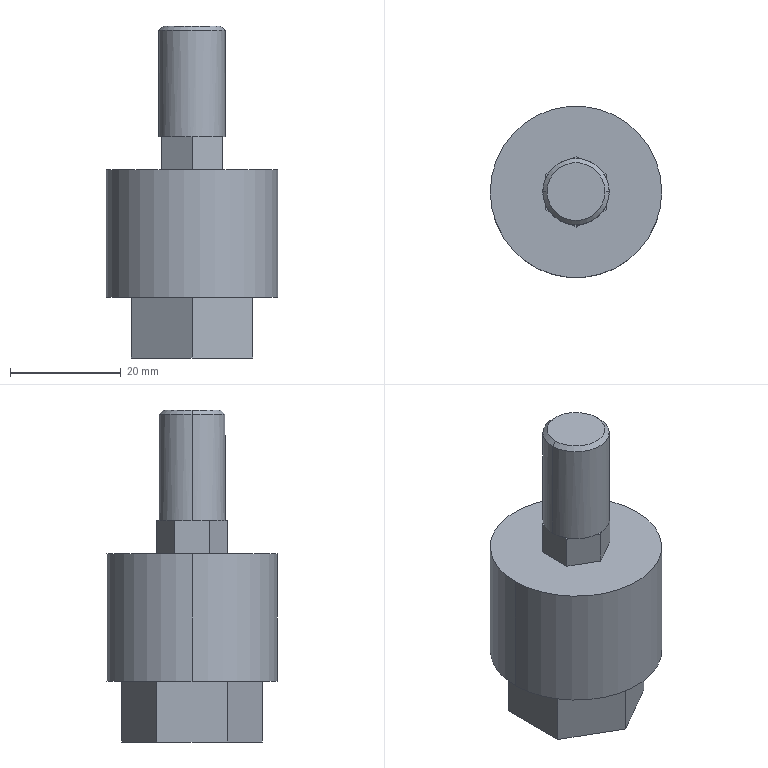Part | STEP file | JA40_12_125_JA40-12-125 | 1 solid | 39 faces | box 31 x 31 x 60 mm | volume 23685 mm3 | plane 29 | cylinder 6 | cone 4 | commonest cylinder face diameters 10.647 x2 12 x2 31 x2
STEP:
#1=CARTESIAN_POINT('',(-6.,0.,59.233));
#2=VERTEX_POINT('',#1);
#3=CARTESIAN_POINT('',(6.,0.,59.233));
#4=VERTEX_POINT('',#3);
#5=CARTESIAN_POINT('',(0.,0.,59.233));
#6=DIRECTION('',(0.,0.,-1.));
#7=DIRECTION('',(-1.,0.,0.));
#8=AXIS2_PLACEMENT_3D('',#5,#6,#7);
#9=CIRCLE('',#8,6.);
#10=EDGE_CURVE('',#2,#4,#9,.T.);
#11=ORIENTED_EDGE('',*,*,#10,.T.);
#12=CARTESIAN_POINT('',(6.,0.,40.));
#13=VERTEX_POINT('',#12);
#14=CARTESIAN_POINT('',(6.,0.,40.));
#15=DIRECTION('',(0.,0.,-1.));
#16=VECTOR('',#15,1000.);
#17=LINE('',#14,#16);
#18=EDGE_CURVE('',#4,#13,#17,.T.);
#19=ORIENTED_EDGE('',*,*,#18,.T.);
#20=CARTESIAN_POINT('',(5.5,2.398,40.));
#21=VERTEX_POINT('',#20);
#22=CARTESIAN_POINT('',(0.,0.,40.));
#23=DIRECTION('',(0.,0.,-1.));
#24=DIRECTION('',(-1.,0.,0.));
#25=AXIS2_PLACEMENT_3D('',#22,#23,#24);
#26=CIRCLE('',#25,6.);
#27=EDGE_CURVE('',#21,#13,#26,.T.);
#28=ORIENTED_EDGE('',*,*,#27,.F.);
#29=CARTESIAN_POINT('',(4.827,3.564,40.));
#30=VERTEX_POINT('',#29);
#31=CARTESIAN_POINT('',(0.,0.,40.));
#32=DIRECTION('',(0.,0.,-1.));
#33=DIRECTION('',(-1.,0.,0.));
#34=AXIS2_PLACEMENT_3D('',#31,#32,#33);
#35=CIRCLE('',#34,6.);
#36=EDGE_CURVE('',#30,#21,#35,.T.);
#37=ORIENTED_EDGE('',*,*,#36,.F.);
#38=CARTESIAN_POINT('',(0.6733,5.962,40.));
#39=VERTEX_POINT('',#38);
#40=CARTESIAN_POINT('',(0.,0.,40.));
#41=DIRECTION('',(0.,0.,-1.));
#42=DIRECTION('',(-1.,0.,0.));
#43=AXIS2_PLACEMENT_3D('',#40,#41,#42);
#44=CIRCLE('',#43,6.);
#45=EDGE_CURVE('',#39,#30,#44,.T.);
#46=ORIENTED_EDGE('',*,*,#45,.F.);
#47=CARTESIAN_POINT('',(-0.6733,5.962,40.));
#48=VERTEX_POINT('',#47);
#49=CARTESIAN_POINT('',(0.,0.,40.));
#50=DIRECTION('',(0.,0.,-1.));
#51=DIRECTION('',(-1.,0.,0.));
#52=AXIS2_PLACEMENT_3D('',#49,#50,#51);
#53=CIRCLE('',#52,6.);
#54=EDGE_CURVE('',#48,#39,#53,.T.);
#55=ORIENTED_EDGE('',*,*,#54,.F.);
#56=CARTESIAN_POINT('',(-4.827,3.564,40.));
#57=VERTEX_POINT('',#56);
#58=CARTESIAN_POINT('',(0.,0.,40.));
#59=DIRECTION('',(0.,0.,-1.));
#60=DIRECTION('',(-1.,0.,0.));
#61=AXIS2_PLACEMENT_3D('',#58,#59,#60);
#62=CIRCLE('',#61,6.);
#63=EDGE_CURVE('',#57,#48,#62,.T.);
#64=ORIENTED_EDGE('',*,*,#63,.F.);
#65=CARTESIAN_POINT('',(-5.5,2.398,40.));
#66=VERTEX_POINT('',#65);
#67=CARTESIAN_POINT('',(0.,0.,40.));
#68=DIRECTION('',(0.,0.,-1.));
#69=DIRECTION('',(-1.,0.,0.));
#70=AXIS2_PLACEMENT_3D('',#67,#68,#69);
#71=CIRCLE('',#70,6.);
#72=EDGE_CURVE('',#66,#57,#71,.T.);
#73=ORIENTED_EDGE('',*,*,#72,.F.);
#74=CARTESIAN_POINT('',(-6.,0.,40.));
#75=VERTEX_POINT('',#74);
#76=CARTESIAN_POINT('',(0.,0.,40.));
#77=DIRECTION('',(0.,0.,-1.));
#78=DIRECTION('',(-1.,0.,0.));
#79=AXIS2_PLACEMENT_3D('',#76,#77,#78);
#80=CIRCLE('',#79,6.);
#81=EDGE_CURVE('',#75,#66,#80,.T.);
#82=ORIENTED_EDGE('',*,*,#81,.F.);
#83=CARTESIAN_POINT('',(-6.,0.,40.));
#84=DIRECTION('',(0.,0.,-1.));
#85=VECTOR('',#84,1000.);
#86=LINE('',#83,#85);
#87=EDGE_CURVE('',#2,#75,#86,.T.);
#88=ORIENTED_EDGE('',*,*,#87,.F.);
#89=EDGE_LOOP('',(#11,#19,#28,#37,#46,#55,#64,#73,#82,#88));
#90=FACE_OUTER_BOUND('',#89,.T.);
#91=CARTESIAN_POINT('',(0.,0.,40.));
#92=DIRECTION('',(0.,0.,-1.));
#93=DIRECTION('',(-1.,0.,0.));
#94=AXIS2_PLACEMENT_3D('',#91,#92,#93);
#95=CYLINDRICAL_SURFACE('',#94,6.);
#96=ADVANCED_FACE('',(#90),#95,.T.);
#97=CARTESIAN_POINT('',(-5.233,0.,60.));
#98=VERTEX_POINT('',#97);
#99=CARTESIAN_POINT('',(5.233,0.,60.));
#100=VERTEX_POINT('',#99);
#101=CARTESIAN_POINT('',(0.,0.,60.));
#102=DIRECTION('',(0.,0.,-1.));
#103=DIRECTION('',(-1.,0.,0.));
#104=AXIS2_PLACEMENT_3D('',#101,#102,#103);
#105=CIRCLE('',#104,5.233);
#106=EDGE_CURVE('',#98,#100,#105,.T.);
#107=ORIENTED_EDGE('',*,*,#106,.T.);
#108=CARTESIAN_POINT('',(6.,0.,59.233));
#109=DIRECTION('',(0.7071,0.,-0.7071));
#110=VECTOR('',#109,1000.);
#111=LINE('',#108,#110);
#112=EDGE_CURVE('',#100,#4,#111,.T.);
#113=ORIENTED_EDGE('',*,*,#112,.T.);
#114=ORIENTED_EDGE('',*,*,#10,.F.);
#115=CARTESIAN_POINT('',(-6.,0.,59.233));
#116=DIRECTION('',(-0.7071,0.,-0.7071));
#117=VECTOR('',#116,1000.);
#118=LINE('',#115,#117);
#119=EDGE_CURVE('',#98,#2,#118,.T.);
#120=ORIENTED_EDGE('',*,*,#119,.F.);
#121=EDGE_LOOP('',(#107,#113,#114,#120));
#122=FACE_OUTER_BOUND('',#121,.T.);
#123=CARTESIAN_POINT('',(0.,0.,59.233));
#124=DIRECTION('',(0.,0.,-1.));
#125=DIRECTION('',(-1.,0.,0.));
#126=AXIS2_PLACEMENT_3D('',#123,#124,#125);
#127=CONICAL_SURFACE('',#126,6.,0.7854);
#128=ADVANCED_FACE('',(#122),#127,.T.);
#129=CARTESIAN_POINT('',(5.324,0.,0.6765));
#130=VERTEX_POINT('',#129);
#131=CARTESIAN_POINT('',(-5.324,0.,0.6765));
#132=VERTEX_POINT('',#131);
#133=CARTESIAN_POINT('',(0.,0.,0.6765));
#134=DIRECTION('',(0.,0.,-1.));
#135=DIRECTION('',(-1.,0.,0.));
#136=AXIS2_PLACEMENT_3D('',#133,#134,#135);
#137=CIRCLE('',#136,5.324);
#138=EDGE_CURVE('',#130,#132,#137,.T.);
#139=ORIENTED_EDGE('',*,*,#138,.F.);
#140=CARTESIAN_POINT('',(6.,0.,0.));
#141=VERTEX_POINT('',#140);
#142=CARTESIAN_POINT('',(5.324,0.,0.6765));
#143=DIRECTION('',(0.7071,0.,-0.7071));
#144=VECTOR('',#143,1000.);
#145=LINE('',#142,#144);
#146=EDGE_CURVE('',#130,#141,#145,.T.);
#147=ORIENTED_EDGE('',*,*,#146,.T.);
#148=CARTESIAN_POINT('',(-6.,0.,0.));
#149=VERTEX_POINT('',#148);
#150=CARTESIAN_POINT('',(0.,0.,0.));
#151=DIRECTION('',(0.,0.,-1.));
#152=DIRECTION('',(-1.,0.,0.));
#153=AXIS2_PLACEMENT_3D('',#150,#151,#152);
#154=CIRCLE('',#153,6.);
#155=EDGE_CURVE('',#141,#149,#154,.T.);
#156=ORIENTED_EDGE('',*,*,#155,.T.);
#157=CARTESIAN_POINT('',(-5.324,0.,0.6765));
#158=DIRECTION('',(-0.7071,0.,-0.7071));
#159=VECTOR('',#158,1000.);
#160=LINE('',#157,#159);
#161=EDGE_CURVE('',#132,#149,#160,.T.);
#162=ORIENTED_EDGE('',*,*,#161,.F.);
#163=EDGE_LOOP('',(#139,#147,#156,#162));
#164=FACE_OUTER_BOUND('',#163,.T.);
#165=CARTESIAN_POINT('',(0.,0.,0.6765));
#166=DIRECTION('',(0.,0.,-1.));
#167=DIRECTION('',(-1.,0.,0.));
#168=AXIS2_PLACEMENT_3D('',#165,#166,#167);
#169=CONICAL_SURFACE('',#168,5.324,0.7854);
#170=ADVANCED_FACE('',(#164),#169,.F.);
#171=CARTESIAN_POINT('',(5.324,0.,13.));
#172=VERTEX_POINT('',#171);
#173=CARTESIAN_POINT('',(-5.324,0.,13.));
#174=VERTEX_POINT('',#173);
#175=CARTESIAN_POINT('',(0.,0.,13.));
#176=DIRECTION('',(0.,0.,-1.));
#177=DIRECTION('',(-1.,0.,0.));
#178=AXIS2_PLACEMENT_3D('',#175,#176,#177);
#179=CIRCLE('',#178,5.324);
#180=EDGE_CURVE('',#172,#174,#179,.T.);
#181=ORIENTED_EDGE('',*,*,#180,.F.);
#182=CARTESIAN_POINT('',(5.324,0.,0.));
#183=DIRECTION('',(0.,0.,-1.));
#184=VECTOR('',#183,1000.);
#185=LINE('',#182,#184);
#186=EDGE_CURVE('',#172,#130,#185,.T.);
#187=ORIENTED_EDGE('',*,*,#186,.T.);
#188=ORIENTED_EDGE('',*,*,#138,.T.);
#189=CARTESIAN_POINT('',(-5.324,0.,0.));
#190=DIRECTION('',(0.,0.,-1.));
#191=VECTOR('',#190,1000.);
#192=LINE('',#189,#191);
#193=EDGE_CURVE('',#174,#132,#192,.T.);
#194=ORIENTED_EDGE('',*,*,#193,.F.);
#195=EDGE_LOOP('',(#181,#187,#188,#194));
#196=FACE_OUTER_BOUND('',#195,.T.);
#197=CARTESIAN_POINT('',(0.,0.,0.));
#198=DIRECTION('',(0.,0.,-1.));
#199=DIRECTION('',(-1.,0.,0.));
#200=AXIS2_PLACEMENT_3D('',#197,#198,#199);
#201=CYLINDRICAL_SURFACE('',#200,5.324);
#202=ADVANCED_FACE('',(#196),#201,.F.);
#203=CARTESIAN_POINT('',(-15.5,0.,34.));
#204=VERTEX_POINT('',#203);
#205=CARTESIAN_POINT('',(15.5,0.,34.));
#206=VERTEX_POINT('',#205);
#207=CARTESIAN_POINT('',(0.,0.,34.));
#208=DIRECTION('',(0.,0.,-1.));
#209=DIRECTION('',(-1.,0.,0.));
#210=AXIS2_PLACEMENT_3D('',#207,#208,#209);
#211=CIRCLE('',#210,15.5);
#212=EDGE_CURVE('',#204,#206,#211,.T.);
#213=ORIENTED_EDGE('',*,*,#212,.T.);
#214=CARTESIAN_POINT('',(15.5,0.,11.));
#215=VERTEX_POINT('',#214);
#216=CARTESIAN_POINT('',(15.5,0.,0.));
#217=DIRECTION('',(0.,0.,-1.));
#218=VECTOR('',#217,1000.);
#219=LINE('',#216,#218);
#220=EDGE_CURVE('',#206,#215,#219,.T.);
#221=ORIENTED_EDGE('',*,*,#220,.T.);
#222=CARTESIAN_POINT('',(-15.5,0.,11.));
#223=VERTEX_POINT('',#222);
#224=CARTESIAN_POINT('',(0.,0.,11.));
#225=DIRECTION('',(0.,0.,-1.));
#226=DIRECTION('',(-1.,0.,0.));
#227=AXIS2_PLACEMENT_3D('',#224,#225,#226);
#228=CIRCLE('',#227,15.5);
#229=EDGE_CURVE('',#223,#215,#228,.T.);
#230=ORIENTED_EDGE('',*,*,#229,.F.);
#231=CARTESIAN_POINT('',(-15.5,0.,0.));
#232=DIRECTION('',(0.,0.,-1.));
#233=VECTOR('',#232,1000.);
#234=LINE('',#231,#233);
#235=EDGE_CURVE('',#204,#223,#234,.T.);
#236=ORIENTED_EDGE('',*,*,#235,.F.);
#237=EDGE_LOOP('',(#213,#221,#230,#236));
#238=FACE_OUTER_BOUND('',#237,.T.);
#239=CARTESIAN_POINT('',(0.,0.,0.));
#240=DIRECTION('',(0.,0.,-1.));
#241=DIRECTION('',(-1.,0.,0.));
#242=AXIS2_PLACEMENT_3D('',#239,#240,#241);
#243=CYLINDRICAL_SURFACE('',#242,15.5);
#244=ADVANCED_FACE('',(#238),#243,.T.);
#245=CARTESIAN_POINT('',(-5.5,3.175,40.));
#246=VERTEX_POINT('',#245);
#247=CARTESIAN_POINT('',(-5.5,3.175,40.));
#248=DIRECTION('',(0.,-1.,0.));
#249=VECTOR('',#248,1000.);
#250=LINE('',#247,#249);
#251=EDGE_CURVE('',#246,#66,#250,.T.);
#252=ORIENTED_EDGE('',*,*,#251,.T.);
#253=ORIENTED_EDGE('',*,*,#72,.T.);
#254=CARTESIAN_POINT('',(0.,6.351,40.));
#255=DIRECTION('',(-0.866,-0.5,0.));
#256=VECTOR('',#255,1000.);
#257=LINE('',#254,#256);
#258=EDGE_CURVE('',#57,#246,#257,.T.);
#259=ORIENTED_EDGE('',*,*,#258,.T.);
#260=EDGE_LOOP('',(#252,#253,#259));
#261=FACE_OUTER_BOUND('',#260,.T.);
#262=CARTESIAN_POINT('',(-5.5,3.175,40.));
#263=DIRECTION('',(0.,0.,1.));
#264=DIRECTION('',(1.,0.,0.));
#265=AXIS2_PLACEMENT_3D('',#262,#263,#264);
#266=PLANE('',#265);
#267=ADVANCED_FACE('',(#261),#266,.T.);
#268=CARTESIAN_POINT('',(0.,6.351,40.));
#269=VERTEX_POINT('',#268);
#270=CARTESIAN_POINT('',(0.,6.351,40.));
#271=DIRECTION('',(-0.866,-0.5,0.));
#272=VECTOR('',#271,1000.);
#273=LINE('',#270,#272);
#274=EDGE_CURVE('',#269,#48,#273,.T.);
#275=ORIENTED_EDGE('',*,*,#274,.T.);
#276=ORIENTED_EDGE('',*,*,#54,.T.);
#277=CARTESIAN_POINT('',(5.5,3.175,40.));
#278=DIRECTION('',(-0.866,0.5,0.));
#279=VECTOR('',#278,1000.);
#280=LINE('',#277,#279);
#281=EDGE_CURVE('',#39,#269,#280,.T.);
#282=ORIENTED_EDGE('',*,*,#281,.T.);
#283=EDGE_LOOP('',(#275,#276,#282));
#284=FACE_OUTER_BOUND('',#283,.T.);
#285=CARTESIAN_POINT('',(-5.5,3.175,40.));
#286=DIRECTION('',(0.,0.,1.));
#287=DIRECTION('',(1.,0.,0.));
#288=AXIS2_PLACEMENT_3D('',#285,#286,#287);
#289=PLANE('',#288);
#290=ADVANCED_FACE('',(#284),#289,.T.);
#291=CARTESIAN_POINT('',(5.5,3.175,40.));
#292=VERTEX_POINT('',#291);
#293=CARTESIAN_POINT('',(5.5,3.175,40.));
#294=DIRECTION('',(-0.866,0.5,0.));
#295=VECTOR('',#294,1000.);
#296=LINE('',#293,#295);
#297=EDGE_CURVE('',#292,#30,#296,.T.);
#298=ORIENTED_EDGE('',*,*,#297,.T.);
#299=ORIENTED_EDGE('',*,*,#36,.T.);
#300=CARTESIAN_POINT('',(5.5,-3.175,40.));
#301=DIRECTION('',(0.,1.,0.));
#302=VECTOR('',#301,1000.);
#303=LINE('',#300,#302);
#304=EDGE_CURVE('',#21,#292,#303,.T.);
#305=ORIENTED_EDGE('',*,*,#304,.T.);
#306=EDGE_LOOP('',(#298,#299,#305));
#307=FACE_OUTER_BOUND('',#306,.T.);
#308=CARTESIAN_POINT('',(-5.5,3.175,40.));
#309=DIRECTION('',(0.,0.,1.));
#310=DIRECTION('',(1.,0.,0.));
#311=AXIS2_PLACEMENT_3D('',#308,#309,#310);
#312=PLANE('',#311);
#313=ADVANCED_FACE('',(#307),#312,.T.);
#314=CARTESIAN_POINT('',(5.5,-3.175,40.));
#315=VERTEX_POINT('',#314);
#316=CARTESIAN_POINT('',(5.5,-2.398,40.));
#317=VERTEX_POINT('',#316);
#318=CARTESIAN_POINT('',(5.5,-3.175,40.));
#319=DIRECTION('',(0.,1.,0.));
#320=VECTOR('',#319,1000.);
#321=LINE('',#318,#320);
#322=EDGE_CURVE('',#315,#317,#321,.T.);
#323=ORIENTED_EDGE('',*,*,#322,.T.);
#324=CARTESIAN_POINT('',(4.827,-3.564,40.));
#325=VERTEX_POINT('',#324);
#326=CARTESIAN_POINT('',(0.,0.,40.));
#327=DIRECTION('',(0.,0.,-1.));
#328=DIRECTION('',(-1.,0.,0.));
#329=AXIS2_PLACEMENT_3D('',#326,#327,#328);
#330=CIRCLE('',#329,6.);
#331=EDGE_CURVE('',#317,#325,#330,.T.);
#332=ORIENTED_EDGE('',*,*,#331,.T.);
#333=CARTESIAN_POINT('',(0.,-6.351,40.));
#334=DIRECTION('',(0.866,0.5,0.));
#335=VECTOR('',#334,1000.);
#336=LINE('',#333,#335);
#337=EDGE_CURVE('',#325,#315,#336,.T.);
#338=ORIENTED_EDGE('',*,*,#337,.T.);
#339=EDGE_LOOP('',(#323,#332,#338));
#340=FACE_OUTER_BOUND('',#339,.T.);
#341=CARTESIAN_POINT('',(-5.5,3.175,40.));
#342=DIRECTION('',(0.,0.,1.));
#343=DIRECTION('',(1.,0.,0.));
#344=AXIS2_PLACEMENT_3D('',#341,#342,#343);
#345=PLANE('',#344);
#346=ADVANCED_FACE('',(#340),#345,.T.);
#347=CARTESIAN_POINT('',(0.,-6.351,40.));
#348=VERTEX_POINT('',#347);
#349=CARTESIAN_POINT('',(0.6733,-5.962,40.));
#350=VERTEX_POINT('',#349);
#351=CARTESIAN_POINT('',(0.,-6.351,40.));
#352=DIRECTION('',(0.866,0.5,0.));
#353=VECTOR('',#352,1000.);
#354=LINE('',#351,#353);
#355=EDGE_CURVE('',#348,#350,#354,.T.);
#356=ORIENTED_EDGE('',*,*,#355,.T.);
#357=CARTESIAN_POINT('',(-0.6733,-5.962,40.));
#358=VERTEX_POINT('',#357);
#359=CARTESIAN_POINT('',(0.,0.,40.));
#360=DIRECTION('',(0.,0.,-1.));
#361=DIRECTION('',(-1.,0.,0.));
#362=AXIS2_PLACEMENT_3D('',#359,#360,#361);
#363=CIRCLE('',#362,6.);
#364=EDGE_CURVE('',#350,#358,#363,.T.);
#365=ORIENTED_EDGE('',*,*,#364,.T.);
#366=CARTESIAN_POINT('',(-5.5,-3.175,40.));
#367=DIRECTION('',(0.866,-0.5,0.));
#368=VECTOR('',#367,1000.);
#369=LINE('',#366,#368);
#370=EDGE_CURVE('',#358,#348,#369,.T.);
#371=ORIENTED_EDGE('',*,*,#370,.T.);
#372=EDGE_LOOP('',(#356,#365,#371));
#373=FACE_OUTER_BOUND('',#372,.T.);
#374=CARTESIAN_POINT('',(-5.5,3.175,40.));
#375=DIRECTION('',(0.,0.,1.));
#376=DIRECTION('',(1.,0.,0.));
#377=AXIS2_PLACEMENT_3D('',#374,#375,#376);
#378=PLANE('',#377);
#379=ADVANCED_FACE('',(#373),#378,.T.);
#380=CARTESIAN_POINT('',(-5.5,-3.175,40.));
#381=VERTEX_POINT('',#380);
#382=CARTESIAN_POINT('',(-4.827,-3.564,40.));
#383=VERTEX_POINT('',#382);
#384=CARTESIAN_POINT('',(-5.5,-3.175,40.));
#385=DIRECTION('',(0.866,-0.5,0.));
#386=VECTOR('',#385,1000.);
#387=LINE('',#384,#386);
#388=EDGE_CURVE('',#381,#383,#387,.T.);
#389=ORIENTED_EDGE('',*,*,#388,.T.);
#390=CARTESIAN_POINT('',(-5.5,-2.398,40.));
#391=VERTEX_POINT('',#390);
#392=CARTESIAN_POINT('',(0.,0.,40.));
#393=DIRECTION('',(0.,0.,-1.));
#394=DIRECTION('',(-1.,0.,0.));
#395=AXIS2_PLACEMENT_3D('',#392,#393,#394);
#396=CIRCLE('',#395,6.);
#397=EDGE_CURVE('',#383,#391,#396,.T.);
#398=ORIENTED_EDGE('',*,*,#397,.T.);
#399=CARTESIAN_POINT('',(-5.5,3.175,40.));
#400=DIRECTION('',(0.,-1.,0.));
#401=VECTOR('',#400,1000.);
#402=LINE('',#399,#401);
#403=EDGE_CURVE('',#391,#381,#402,.T.);
#404=ORIENTED_EDGE('',*,*,#403,.T.);
#405=EDGE_LOOP('',(#389,#398,#404));
#406=FACE_OUTER_BOUND('',#405,.T.);
#407=CARTESIAN_POINT('',(-5.5,3.175,40.));
#408=DIRECTION('',(0.,0.,1.));
#409=DIRECTION('',(1.,0.,0.));
#410=AXIS2_PLACEMENT_3D('',#407,#408,#409);
#411=PLANE('',#410);
#412=ADVANCED_FACE('',(#406),#411,.T.);
#413=ORIENTED_EDGE('',*,*,#274,.F.);
#414=CARTESIAN_POINT('',(0.,6.351,34.));
#415=VERTEX_POINT('',#414);
#416=CARTESIAN_POINT('',(0.,6.351,34.));
#417=DIRECTION('',(0.,0.,1.));
#418=VECTOR('',#417,1000.);
#419=LINE('',#416,#418);
#420=EDGE_CURVE('',#415,#269,#419,.T.);
#421=ORIENTED_EDGE('',*,*,#420,.F.);
#422=CARTESIAN_POINT('',(-5.5,3.175,34.));
#423=VERTEX_POINT('',#422);
#424=CARTESIAN_POINT('',(0.,6.351,34.));
#425=DIRECTION('',(-0.866,-0.5,0.));
#426=VECTOR('',#425,1000.);
#427=LINE('',#424,#426);
#428=EDGE_CURVE('',#415,#423,#427,.T.);
#429=ORIENTED_EDGE('',*,*,#428,.T.);
#430=CARTESIAN_POINT('',(-5.5,3.175,34.));
#431=DIRECTION('',(0.,0.,1.));
#432=VECTOR('',#431,1000.);
#433=LINE('',#430,#432);
#434=EDGE_CURVE('',#423,#246,#433,.T.);
#435=ORIENTED_EDGE('',*,*,#434,.T.);
#436=ORIENTED_EDGE('',*,*,#258,.F.);
#437=CARTESIAN_POINT('',(0.,6.351,40.));
#438=DIRECTION('',(-0.866,-0.5,0.));
#439=VECTOR('',#438,1000.);
#440=LINE('',#437,#439);
#441=EDGE_CURVE('',#48,#57,#440,.T.);
#442=ORIENTED_EDGE('',*,*,#441,.F.);
#443=EDGE_LOOP('',(#413,#421,#429,#435,#436,#442));
#444=FACE_OUTER_BOUND('',#443,.T.);
#445=CARTESIAN_POINT('',(0.,6.351,34.));
#446=DIRECTION('',(-0.5,0.866,0.));
#447=DIRECTION('',(-0.866,-0.5,0.));
#448=AXIS2_PLACEMENT_3D('',#445,#446,#447);
#449=PLANE('',#448);
#450=ADVANCED_FACE('',(#444),#449,.T.);
#451=ORIENTED_EDGE('',*,*,#297,.F.);
#452=CARTESIAN_POINT('',(5.5,3.175,34.));
#453=VERTEX_POINT('',#452);
#454=CARTESIAN_POINT('',(5.5,3.175,34.));
#455=DIRECTION('',(0.,0.,1.));
#456=VECTOR('',#455,1000.);
#457=LINE('',#454,#456);
#458=EDGE_CURVE('',#453,#292,#457,.T.);
#459=ORIENTED_EDGE('',*,*,#458,.F.);
#460=CARTESIAN_POINT('',(5.5,3.175,34.));
#461=DIRECTION('',(-0.866,0.5,0.));
#462=VECTOR('',#461,1000.);
#463=LINE('',#460,#462);
#464=EDGE_CURVE('',#453,#415,#463,.T.);
#465=ORIENTED_EDGE('',*,*,#464,.T.);
#466=ORIENTED_EDGE('',*,*,#420,.T.);
#467=ORIENTED_EDGE('',*,*,#281,.F.);
#468=CARTESIAN_POINT('',(5.5,3.175,40.));
#469=DIRECTION('',(-0.866,0.5,0.));
#470=VECTOR('',#469,1000.);
#471=LINE('',#468,#470);
#472=EDGE_CURVE('',#30,#39,#471,.T.);
#473=ORIENTED_EDGE('',*,*,#472,.F.);
#474=EDGE_LOOP('',(#451,#459,#465,#466,#467,#473));
#475=FACE_OUTER_BOUND('',#474,.T.);
#476=CARTESIAN_POINT('',(5.5,3.175,34.));
#477=DIRECTION('',(0.5,0.866,0.));
#478=DIRECTION('',(-0.866,0.5,0.));
#479=AXIS2_PLACEMENT_3D('',#476,#477,#478);
#480=PLANE('',#479);
#481=ADVANCED_FACE('',(#475),#480,.T.);
#482=ORIENTED_EDGE('',*,*,#322,.F.);
#483=CARTESIAN_POINT('',(5.5,-3.175,34.));
#484=VERTEX_POINT('',#483);
#485=CARTESIAN_POINT('',(5.5,-3.175,34.));
#486=DIRECTION('',(0.,0.,1.));
#487=VECTOR('',#486,1000.);
#488=LINE('',#485,#487);
#489=EDGE_CURVE('',#484,#315,#488,.T.);
#490=ORIENTED_EDGE('',*,*,#489,.F.);
#491=CARTESIAN_POINT('',(5.5,-3.175,34.));
#492=DIRECTION('',(0.,1.,0.));
#493=VECTOR('',#492,1000.);
#494=LINE('',#491,#493);
#495=EDGE_CURVE('',#484,#453,#494,.T.);
#496=ORIENTED_EDGE('',*,*,#495,.T.);
#497=ORIENTED_EDGE('',*,*,#458,.T.);
#498=ORIENTED_EDGE('',*,*,#304,.F.);
#499=CARTESIAN_POINT('',(5.5,-3.175,40.));
#500=DIRECTION('',(0.,1.,0.));
#501=VECTOR('',#500,1000.);
#502=LINE('',#499,#501);
#503=EDGE_CURVE('',#317,#21,#502,.T.);
#504=ORIENTED_EDGE('',*,*,#503,.F.);
#505=EDGE_LOOP('',(#482,#490,#496,#497,#498,#504));
#506=FACE_OUTER_BOUND('',#505,.T.);
#507=CARTESIAN_POINT('',(5.5,-3.175,34.));
#508=DIRECTION('',(1.,0.,0.));
#509=DIRECTION('',(0.,0.,-1.));
#510=AXIS2_PLACEMENT_3D('',#507,#508,#509);
#511=PLANE('',#510);
#512=ADVANCED_FACE('',(#506),#511,.T.);
#513=ORIENTED_EDGE('',*,*,#355,.F.);
#514=CARTESIAN_POINT('',(0.,-6.351,34.));
#515=VERTEX_POINT('',#514);
#516=CARTESIAN_POINT('',(0.,-6.351,34.));
#517=DIRECTION('',(0.,0.,1.));
#518=VECTOR('',#517,1000.);
#519=LINE('',#516,#518);
#520=EDGE_CURVE('',#515,#348,#519,.T.);
#521=ORIENTED_EDGE('',*,*,#520,.F.);
#522=CARTESIAN_POINT('',(0.,-6.351,34.));
#523=DIRECTION('',(0.866,0.5,0.));
#524=VECTOR('',#523,1000.);
#525=LINE('',#522,#524);
#526=EDGE_CURVE('',#515,#484,#525,.T.);
#527=ORIENTED_EDGE('',*,*,#526,.T.);
#528=ORIENTED_EDGE('',*,*,#489,.T.);
#529=ORIENTED_EDGE('',*,*,#337,.F.);
#530=CARTESIAN_POINT('',(0.,-6.351,40.));
#531=DIRECTION('',(0.866,0.5,0.));
#532=VECTOR('',#531,1000.);
#533=LINE('',#530,#532);
#534=EDGE_CURVE('',#350,#325,#533,.T.);
#535=ORIENTED_EDGE('',*,*,#534,.F.);
#536=EDGE_LOOP('',(#513,#521,#527,#528,#529,#535));
#537=FACE_OUTER_BOUND('',#536,.T.);
#538=CARTESIAN_POINT('',(0.,-6.351,34.));
#539=DIRECTION('',(0.5,-0.866,0.));
#540=DIRECTION('',(0.866,0.5,0.));
#541=AXIS2_PLACEMENT_3D('',#538,#539,#540);
#542=PLANE('',#541);
#543=ADVANCED_FACE('',(#537),#542,.T.);
#544=ORIENTED_EDGE('',*,*,#388,.F.);
#545=CARTESIAN_POINT('',(-5.5,-3.175,34.));
#546=VERTEX_POINT('',#545);
#547=CARTESIAN_POINT('',(-5.5,-3.175,34.));
#548=DIRECTION('',(0.,0.,1.));
#549=VECTOR('',#548,1000.);
#550=LINE('',#547,#549);
#551=EDGE_CURVE('',#546,#381,#550,.T.);
#552=ORIENTED_EDGE('',*,*,#551,.F.);
#553=CARTESIAN_POINT('',(-5.5,-3.175,34.));
#554=DIRECTION('',(0.866,-0.5,0.));
#555=VECTOR('',#554,1000.);
#556=LINE('',#553,#555);
#557=EDGE_CURVE('',#546,#515,#556,.T.);
#558=ORIENTED_EDGE('',*,*,#557,.T.);
#559=ORIENTED_EDGE('',*,*,#520,.T.);
#560=ORIENTED_EDGE('',*,*,#370,.F.);
#561=CARTESIAN_POINT('',(-5.5,-3.175,40.));
#562=DIRECTION('',(0.866,-0.5,0.));
#563=VECTOR('',#562,1000.);
#564=LINE('',#561,#563);
#565=EDGE_CURVE('',#383,#358,#564,.T.);
#566=ORIENTED_EDGE('',*,*,#565,.F.);
#567=EDGE_LOOP('',(#544,#552,#558,#559,#560,#566));
#568=FACE_OUTER_BOUND('',#567,.T.);
#569=CARTESIAN_POINT('',(-5.5,-3.175,34.));
#570=DIRECTION('',(-0.5,-0.866,0.));
#571=DIRECTION('',(0.866,-0.5,0.));
#572=AXIS2_PLACEMENT_3D('',#569,#570,#571);
#573=PLANE('',#572);
#574=ADVANCED_FACE('',(#568),#573,.T.);
#575=ORIENTED_EDGE('',*,*,#251,.F.);
#576=ORIENTED_EDGE('',*,*,#434,.F.);
#577=CARTESIAN_POINT('',(-5.5,3.175,34.));
#578=DIRECTION('',(0.,-1.,0.));
#579=VECTOR('',#578,1000.);
#580=LINE('',#577,#579);
#581=EDGE_CURVE('',#423,#546,#580,.T.);
#582=ORIENTED_EDGE('',*,*,#581,.T.);
#583=ORIENTED_EDGE('',*,*,#551,.T.);
#584=ORIENTED_EDGE('',*,*,#403,.F.);
#585=CARTESIAN_POINT('',(-5.5,3.175,40.));
#586=DIRECTION('',(0.,-1.,0.));
#587=VECTOR('',#586,1000.);
#588=LINE('',#585,#587);
#589=EDGE_CURVE('',#66,#391,#588,.T.);
#590=ORIENTED_EDGE('',*,*,#589,.F.);
#591=EDGE_LOOP('',(#575,#576,#582,#583,#584,#590));
#592=FACE_OUTER_BOUND('',#591,.T.);
#593=CARTESIAN_POINT('',(-5.5,3.175,34.));
#594=DIRECTION('',(-1.,0.,0.));
#595=DIRECTION('',(0.,0.,1.));
#596=AXIS2_PLACEMENT_3D('',#593,#594,#595);
#597=PLANE('',#596);
#598=ADVANCED_FACE('',(#592),#597,.T.);
#599=ORIENTED_EDGE('',*,*,#581,.F.);
#600=ORIENTED_EDGE('',*,*,#428,.F.);
#601=ORIENTED_EDGE('',*,*,#464,.F.);
#602=ORIENTED_EDGE('',*,*,#495,.F.);
#603=ORIENTED_EDGE('',*,*,#526,.F.);
#604=ORIENTED_EDGE('',*,*,#557,.F.);
#605=EDGE_LOOP('',(#599,#600,#601,#602,#603,#604));
#606=FACE_BOUND('',#605,.T.);
#607=ORIENTED_EDGE('',*,*,#212,.F.);
#608=CARTESIAN_POINT('',(0.,0.,34.));
#609=DIRECTION('',(0.,0.,-1.));
#610=DIRECTION('',(-1.,0.,0.));
#611=AXIS2_PLACEMENT_3D('',#608,#609,#610);
#612=CIRCLE('',#611,15.5);
#613=EDGE_CURVE('',#206,#204,#612,.T.);
#614=ORIENTED_EDGE('',*,*,#613,.F.);
#615=EDGE_LOOP('',(#607,#614));
#616=FACE_OUTER_BOUND('',#615,.T.);
#617=CARTESIAN_POINT('',(0.,0.,34.));
#618=DIRECTION('',(0.,0.,1.));
#619=DIRECTION('',(1.,0.,0.));
#620=AXIS2_PLACEMENT_3D('',#617,#618,#619);
#621=PLANE('',#620);
#622=ADVANCED_FACE('',(#606,#616),#621,.T.);
#623=ORIENTED_EDGE('',*,*,#220,.F.);
#624=ORIENTED_EDGE('',*,*,#613,.T.);
#625=ORIENTED_EDGE('',*,*,#235,.T.);
#626=CARTESIAN_POINT('',(0.,0.,11.));
#627=DIRECTION('',(0.,0.,-1.));
#628=DIRECTION('',(-1.,0.,0.));
#629=AXIS2_PLACEMENT_3D('',#626,#627,#628);
#630=CIRCLE('',#629,15.5);
#631=EDGE_CURVE('',#215,#223,#630,.T.);
#632=ORIENTED_EDGE('',*,*,#631,.F.);
#633=EDGE_LOOP('',(#623,#624,#625,#632));
#634=FACE_OUTER_BOUND('',#633,.T.);
#635=CARTESIAN_POINT('',(0.,0.,0.));
#636=DIRECTION('',(0.,0.,-1.));
#637=DIRECTION('',(-1.,0.,0.));
#638=AXIS2_PLACEMENT_3D('',#635,#636,#637);
#639=CYLINDRICAL_SURFACE('',#638,15.5);
#640=ADVANCED_FACE('',(#634),#639,.T.);
#641=ORIENTED_EDGE('',*,*,#229,.T.);
#642=ORIENTED_EDGE('',*,*,#631,.T.);
#643=EDGE_LOOP('',(#641,#642));
#644=FACE_OUTER_BOUND('',#643,.T.);
#645=CARTESIAN_POINT('',(-11.,6.351,11.));
#646=VERTEX_POINT('',#645);
#647=CARTESIAN_POINT('',(-11.,-6.351,11.));
#648=VERTEX_POINT('',#647);
#649=CARTESIAN_POINT('',(-11.,6.351,11.));
#650=DIRECTION('',(0.,-1.,0.));
#651=VECTOR('',#650,1000.);
#652=LINE('',#649,#651);
#653=EDGE_CURVE('',#646,#648,#652,.T.);
#654=ORIENTED_EDGE('',*,*,#653,.T.);
#655=CARTESIAN_POINT('',(0.,-12.702,11.));
#656=VERTEX_POINT('',#655);
#657=CARTESIAN_POINT('',(-11.,-6.351,11.));
#658=DIRECTION('',(0.866,-0.5,0.));
#659=VECTOR('',#658,1000.);
#660=LINE('',#657,#659);
#661=EDGE_CURVE('',#648,#656,#660,.T.);
#662=ORIENTED_EDGE('',*,*,#661,.T.);
#663=CARTESIAN_POINT('',(11.,-6.351,11.));
#664=VERTEX_POINT('',#663);
#665=CARTESIAN_POINT('',(0.,-12.702,11.));
#666=DIRECTION('',(0.866,0.5,0.));
#667=VECTOR('',#666,1000.);
#668=LINE('',#665,#667);
#669=EDGE_CURVE('',#656,#664,#668,.T.);
#670=ORIENTED_EDGE('',*,*,#669,.T.);
#671=CARTESIAN_POINT('',(11.,6.351,11.));
#672=VERTEX_POINT('',#671);
#673=CARTESIAN_POINT('',(11.,-6.351,11.));
#674=DIRECTION('',(0.,1.,0.));
#675=VECTOR('',#674,1000.);
#676=LINE('',#673,#675);
#677=EDGE_CURVE('',#664,#672,#676,.T.);
#678=ORIENTED_EDGE('',*,*,#677,.T.);
#679=CARTESIAN_POINT('',(0.,12.702,11.));
#680=VERTEX_POINT('',#679);
#681=CARTESIAN_POINT('',(11.,6.351,11.));
#682=DIRECTION('',(-0.866,0.5,0.));
#683=VECTOR('',#682,1000.);
#684=LINE('',#681,#683);
#685=EDGE_CURVE('',#672,#680,#684,.T.);
#686=ORIENTED_EDGE('',*,*,#685,.T.);
#687=CARTESIAN_POINT('',(0.,12.702,11.));
#688=DIRECTION('',(-0.866,-0.5,0.));
#689=VECTOR('',#688,1000.);
#690=LINE('',#687,#689);
#691=EDGE_CURVE('',#680,#646,#690,.T.);
#692=ORIENTED_EDGE('',*,*,#691,.T.);
#693=EDGE_LOOP('',(#654,#662,#670,#678,#686,#692));
#694=FACE_BOUND('',#693,.T.);
#695=CARTESIAN_POINT('',(0.,15.5,11.));
#696=DIRECTION('',(0.,0.,-1.));
#697=DIRECTION('',(-1.,0.,0.));
#698=AXIS2_PLACEMENT_3D('',#695,#696,#697);
#699=PLANE('',#698);
#700=ADVANCED_FACE('',(#644,#694),#699,.T.);
#701=CARTESIAN_POINT('',(0.,12.702,0.));
#702=VERTEX_POINT('',#701);
#703=CARTESIAN_POINT('',(-11.,6.351,0.));
#704=VERTEX_POINT('',#703);
#705=CARTESIAN_POINT('',(0.,12.702,0.));
#706=DIRECTION('',(-0.866,-0.5,0.));
#707=VECTOR('',#706,1000.);
#708=LINE('',#705,#707);
#709=EDGE_CURVE('',#702,#704,#708,.T.);
#710=ORIENTED_EDGE('',*,*,#709,.T.);
#711=CARTESIAN_POINT('',(-11.,6.351,11.));
#712=DIRECTION('',(0.,0.,-1.));
#713=VECTOR('',#712,1000.);
#714=LINE('',#711,#713);
#715=EDGE_CURVE('',#646,#704,#714,.T.);
#716=ORIENTED_EDGE('',*,*,#715,.F.);
#717=ORIENTED_EDGE('',*,*,#691,.F.);
#718=CARTESIAN_POINT('',(0.,12.702,11.));
#719=DIRECTION('',(0.,0.,-1.));
#720=VECTOR('',#719,1000.);
#721=LINE('',#718,#720);
#722=EDGE_CURVE('',#680,#702,#721,.T.);
#723=ORIENTED_EDGE('',*,*,#722,.T.);
#724=EDGE_LOOP('',(#710,#716,#717,#723));
#725=FACE_OUTER_BOUND('',#724,.T.);
#726=CARTESIAN_POINT('',(0.,12.702,11.));
#727=DIRECTION('',(0.5,-0.866,0.));
#728=DIRECTION('',(0.866,0.5,0.));
#729=AXIS2_PLACEMENT_3D('',#726,#727,#728);
#730=PLANE('',#729);
#731=ADVANCED_FACE('',(#725),#730,.F.);
#732=CARTESIAN_POINT('',(-11.,-6.351,0.));
#733=VERTEX_POINT('',#732);
#734=CARTESIAN_POINT('',(-11.,6.351,0.));
#735=DIRECTION('',(0.,-1.,0.));
#736=VECTOR('',#735,1000.);
#737=LINE('',#734,#736);
#738=EDGE_CURVE('',#704,#733,#737,.T.);
#739=ORIENTED_EDGE('',*,*,#738,.T.);
#740=CARTESIAN_POINT('',(-11.,-6.351,11.));
#741=DIRECTION('',(0.,0.,-1.));
#742=VECTOR('',#741,1000.);
#743=LINE('',#740,#742);
#744=EDGE_CURVE('',#648,#733,#743,.T.);
#745=ORIENTED_EDGE('',*,*,#744,.F.);
#746=ORIENTED_EDGE('',*,*,#653,.F.);
#747=ORIENTED_EDGE('',*,*,#715,.T.);
#748=EDGE_LOOP('',(#739,#745,#746,#747));
#749=FACE_OUTER_BOUND('',#748,.T.);
#750=CARTESIAN_POINT('',(-11.,6.351,11.));
#751=DIRECTION('',(1.,0.,0.));
#752=DIRECTION('',(0.,0.,-1.));
#753=AXIS2_PLACEMENT_3D('',#750,#751,#752);
#754=PLANE('',#753);
#755=ADVANCED_FACE('',(#749),#754,.F.);
#756=CARTESIAN_POINT('',(0.,-12.702,0.));
#757=VERTEX_POINT('',#756);
#758=CARTESIAN_POINT('',(-11.,-6.351,0.));
#759=DIRECTION('',(0.866,-0.5,0.));
#760=VECTOR('',#759,1000.);
#761=LINE('',#758,#760);
#762=EDGE_CURVE('',#733,#757,#761,.T.);
#763=ORIENTED_EDGE('',*,*,#762,.T.);
#764=CARTESIAN_POINT('',(0.,-12.702,11.));
#765=DIRECTION('',(0.,0.,-1.));
#766=VECTOR('',#765,1000.);
#767=LINE('',#764,#766);
#768=EDGE_CURVE('',#656,#757,#767,.T.);
#769=ORIENTED_EDGE('',*,*,#768,.F.);
#770=ORIENTED_EDGE('',*,*,#661,.F.);
#771=ORIENTED_EDGE('',*,*,#744,.T.);
#772=EDGE_LOOP('',(#763,#769,#770,#771));
#773=FACE_OUTER_BOUND('',#772,.T.);
#774=CARTESIAN_POINT('',(-11.,-6.351,11.));
#775=DIRECTION('',(0.5,0.866,0.));
#776=DIRECTION('',(-0.866,0.5,0.));
#777=AXIS2_PLACEMENT_3D('',#774,#775,#776);
#778=PLANE('',#777);
#779=ADVANCED_FACE('',(#773),#778,.F.);
#780=CARTESIAN_POINT('',(11.,-6.351,0.));
#781=VERTEX_POINT('',#780);
#782=CARTESIAN_POINT('',(0.,-12.702,0.));
#783=DIRECTION('',(0.866,0.5,0.));
#784=VECTOR('',#783,1000.);
#785=LINE('',#782,#784);
#786=EDGE_CURVE('',#757,#781,#785,.T.);
#787=ORIENTED_EDGE('',*,*,#786,.T.);
#788=CARTESIAN_POINT('',(11.,-6.351,11.));
#789=DIRECTION('',(0.,0.,-1.));
#790=VECTOR('',#789,1000.);
#791=LINE('',#788,#790);
#792=EDGE_CURVE('',#664,#781,#791,.T.);
#793=ORIENTED_EDGE('',*,*,#792,.F.);
#794=ORIENTED_EDGE('',*,*,#669,.F.);
#795=ORIENTED_EDGE('',*,*,#768,.T.);
#796=EDGE_LOOP('',(#787,#793,#794,#795));
#797=FACE_OUTER_BOUND('',#796,.T.);
#798=CARTESIAN_POINT('',(0.,-12.702,11.));
#799=DIRECTION('',(-0.5,0.866,0.));
#800=DIRECTION('',(-0.866,-0.5,0.));
#801=AXIS2_PLACEMENT_3D('',#798,#799,#800);
#802=PLANE('',#801);
#803=ADVANCED_FACE('',(#797),#802,.F.);
#804=CARTESIAN_POINT('',(11.,6.351,0.));
#805=VERTEX_POINT('',#804);
#806=CARTESIAN_POINT('',(11.,-6.351,0.));
#807=DIRECTION('',(0.,1.,0.));
#808=VECTOR('',#807,1000.);
#809=LINE('',#806,#808);
#810=EDGE_CURVE('',#781,#805,#809,.T.);
#811=ORIENTED_EDGE('',*,*,#810,.T.);
#812=CARTESIAN_POINT('',(11.,6.351,11.));
#813=DIRECTION('',(0.,0.,-1.));
#814=VECTOR('',#813,1000.);
#815=LINE('',#812,#814);
#816=EDGE_CURVE('',#672,#805,#815,.T.);
#817=ORIENTED_EDGE('',*,*,#816,.F.);
#818=ORIENTED_EDGE('',*,*,#677,.F.);
#819=ORIENTED_EDGE('',*,*,#792,.T.);
#820=EDGE_LOOP('',(#811,#817,#818,#819));
#821=FACE_OUTER_BOUND('',#820,.T.);
#822=CARTESIAN_POINT('',(11.,-6.351,11.));
#823=DIRECTION('',(-1.,0.,0.));
#824=DIRECTION('',(0.,0.,1.));
#825=AXIS2_PLACEMENT_3D('',#822,#823,#824);
#826=PLANE('',#825);
#827=ADVANCED_FACE('',(#821),#826,.F.);
#828=CARTESIAN_POINT('',(11.,6.351,0.));
#829=DIRECTION('',(-0.866,0.5,0.));
#830=VECTOR('',#829,1000.);
#831=LINE('',#828,#830);
#832=EDGE_CURVE('',#805,#702,#831,.T.);
#833=ORIENTED_EDGE('',*,*,#832,.T.);
#834=ORIENTED_EDGE('',*,*,#722,.F.);
#835=ORIENTED_EDGE('',*,*,#685,.F.);
#836=ORIENTED_EDGE('',*,*,#816,.T.);
#837=EDGE_LOOP('',(#833,#834,#835,#836));
#838=FACE_OUTER_BOUND('',#837,.T.);
#839=CARTESIAN_POINT('',(11.,6.351,11.));
#840=DIRECTION('',(-0.5,-0.866,0.));
#841=DIRECTION('',(0.866,-0.5,0.));
#842=AXIS2_PLACEMENT_3D('',#839,#840,#841);
#843=PLANE('',#842);
#844=ADVANCED_FACE('',(#838),#843,.F.);
#845=CARTESIAN_POINT('',(0.,0.,13.));
#846=DIRECTION('',(0.,0.,-1.));
#847=DIRECTION('',(-1.,0.,0.));
#848=AXIS2_PLACEMENT_3D('',#845,#846,#847);
#849=CIRCLE('',#848,5.324);
#850=EDGE_CURVE('',#174,#172,#849,.T.);
#851=ORIENTED_EDGE('',*,*,#850,.T.);
#852=ORIENTED_EDGE('',*,*,#180,.T.);
#853=EDGE_LOOP('',(#851,#852));
#854=FACE_OUTER_BOUND('',#853,.T.);
#855=CARTESIAN_POINT('',(0.,5.324,13.));
#856=DIRECTION('',(0.,0.,-1.));
#857=DIRECTION('',(-1.,0.,0.));
#858=AXIS2_PLACEMENT_3D('',#855,#856,#857);
#859=PLANE('',#858);
#860=ADVANCED_FACE('',(#854),#859,.T.);
#861=ORIENTED_EDGE('',*,*,#186,.F.);
#862=ORIENTED_EDGE('',*,*,#850,.F.);
#863=ORIENTED_EDGE('',*,*,#193,.T.);
#864=CARTESIAN_POINT('',(0.,0.,0.6765));
#865=DIRECTION('',(0.,0.,-1.));
#866=DIRECTION('',(-1.,0.,0.));
#867=AXIS2_PLACEMENT_3D('',#864,#865,#866);
#868=CIRCLE('',#867,5.324);
#869=EDGE_CURVE('',#132,#130,#868,.T.);
#870=ORIENTED_EDGE('',*,*,#869,.T.);
#871=EDGE_LOOP('',(#861,#862,#863,#870));
#872=FACE_OUTER_BOUND('',#871,.T.);
#873=CARTESIAN_POINT('',(0.,0.,0.));
#874=DIRECTION('',(0.,0.,-1.));
#875=DIRECTION('',(-1.,0.,0.));
#876=AXIS2_PLACEMENT_3D('',#873,#874,#875);
#877=CYLINDRICAL_SURFACE('',#876,5.324);
#878=ADVANCED_FACE('',(#872),#877,.F.);
#879=ORIENTED_EDGE('',*,*,#146,.F.);
#880=ORIENTED_EDGE('',*,*,#869,.F.);
#881=ORIENTED_EDGE('',*,*,#161,.T.);
#882=CARTESIAN_POINT('',(0.,0.,0.));
#883=DIRECTION('',(0.,0.,-1.));
#884=DIRECTION('',(-1.,0.,0.));
#885=AXIS2_PLACEMENT_3D('',#882,#883,#884);
#886=CIRCLE('',#885,6.);
#887=EDGE_CURVE('',#149,#141,#886,.T.);
#888=ORIENTED_EDGE('',*,*,#887,.T.);
#889=EDGE_LOOP('',(#879,#880,#881,#888));
#890=FACE_OUTER_BOUND('',#889,.T.);
#891=CARTESIAN_POINT('',(0.,0.,0.6765));
#892=DIRECTION('',(0.,0.,-1.));
#893=DIRECTION('',(-1.,0.,0.));
#894=AXIS2_PLACEMENT_3D('',#891,#892,#893);
#895=CONICAL_SURFACE('',#894,5.324,0.7854);
#896=ADVANCED_FACE('',(#890),#895,.F.);
#897=ORIENTED_EDGE('',*,*,#709,.F.);
#898=ORIENTED_EDGE('',*,*,#832,.F.);
#899=ORIENTED_EDGE('',*,*,#810,.F.);
#900=ORIENTED_EDGE('',*,*,#786,.F.);
#901=ORIENTED_EDGE('',*,*,#762,.F.);
#902=ORIENTED_EDGE('',*,*,#738,.F.);
#903=EDGE_LOOP('',(#897,#898,#899,#900,#901,#902));
#904=FACE_OUTER_BOUND('',#903,.T.);
#905=ORIENTED_EDGE('',*,*,#887,.F.);
#906=ORIENTED_EDGE('',*,*,#155,.F.);
#907=EDGE_LOOP('',(#905,#906));
#908=FACE_BOUND('',#907,.T.);
#909=CARTESIAN_POINT('',(0.,13.2,0.));
#910=DIRECTION('',(0.,0.,-1.));
#911=DIRECTION('',(-1.,0.,0.));
#912=AXIS2_PLACEMENT_3D('',#909,#910,#911);
#913=PLANE('',#912);
#914=ADVANCED_FACE('',(#904,#908),#913,.T.);
#915=ORIENTED_EDGE('',*,*,#63,.T.);
#916=ORIENTED_EDGE('',*,*,#441,.T.);
#917=EDGE_LOOP('',(#915,#916));
#918=FACE_OUTER_BOUND('',#917,.T.);
#919=CARTESIAN_POINT('',(0.,6.,40.));
#920=DIRECTION('',(0.,0.,-1.));
#921=DIRECTION('',(-1.,0.,0.));
#922=AXIS2_PLACEMENT_3D('',#919,#920,#921);
#923=PLANE('',#922);
#924=ADVANCED_FACE('',(#918),#923,.T.);
#925=CARTESIAN_POINT('',(0.,0.,40.));
#926=DIRECTION('',(0.,0.,-1.));
#927=DIRECTION('',(-1.,0.,0.));
#928=AXIS2_PLACEMENT_3D('',#925,#926,#927);
#929=CIRCLE('',#928,6.);
#930=EDGE_CURVE('',#391,#75,#929,.T.);
#931=ORIENTED_EDGE('',*,*,#930,.T.);
#932=ORIENTED_EDGE('',*,*,#81,.T.);
#933=ORIENTED_EDGE('',*,*,#589,.T.);
#934=EDGE_LOOP('',(#931,#932,#933));
#935=FACE_OUTER_BOUND('',#934,.T.);
#936=CARTESIAN_POINT('',(0.,6.,40.));
#937=DIRECTION('',(0.,0.,-1.));
#938=DIRECTION('',(-1.,0.,0.));
#939=AXIS2_PLACEMENT_3D('',#936,#937,#938);
#940=PLANE('',#939);
#941=ADVANCED_FACE('',(#935),#940,.T.);
#942=CARTESIAN_POINT('',(0.,0.,40.));
#943=DIRECTION('',(0.,0.,-1.));
#944=DIRECTION('',(-1.,0.,0.));
#945=AXIS2_PLACEMENT_3D('',#942,#943,#944);
#946=CIRCLE('',#945,6.);
#947=EDGE_CURVE('',#358,#383,#946,.T.);
#948=ORIENTED_EDGE('',*,*,#947,.T.);
#949=ORIENTED_EDGE('',*,*,#565,.T.);
#950=EDGE_LOOP('',(#948,#949));
#951=FACE_OUTER_BOUND('',#950,.T.);
#952=CARTESIAN_POINT('',(0.,6.,40.));
#953=DIRECTION('',(0.,0.,-1.));
#954=DIRECTION('',(-1.,0.,0.));
#955=AXIS2_PLACEMENT_3D('',#952,#953,#954);
#956=PLANE('',#955);
#957=ADVANCED_FACE('',(#951),#956,.T.);
#958=CARTESIAN_POINT('',(0.,0.,40.));
#959=DIRECTION('',(0.,0.,-1.));
#960=DIRECTION('',(-1.,0.,0.));
#961=AXIS2_PLACEMENT_3D('',#958,#959,#960);
#962=CIRCLE('',#961,6.);
#963=EDGE_CURVE('',#325,#350,#962,.T.);
#964=ORIENTED_EDGE('',*,*,#963,.T.);
#965=ORIENTED_EDGE('',*,*,#534,.T.);
#966=EDGE_LOOP('',(#964,#965));
#967=FACE_OUTER_BOUND('',#966,.T.);
#968=CARTESIAN_POINT('',(0.,6.,40.));
#969=DIRECTION('',(0.,0.,-1.));
#970=DIRECTION('',(-1.,0.,0.));
#971=AXIS2_PLACEMENT_3D('',#968,#969,#970);
#972=PLANE('',#971);
#973=ADVANCED_FACE('',(#967),#972,.T.);
#974=ORIENTED_EDGE('',*,*,#27,.T.);
#975=CARTESIAN_POINT('',(0.,0.,40.));
#976=DIRECTION('',(0.,0.,-1.));
#977=DIRECTION('',(-1.,0.,0.));
#978=AXIS2_PLACEMENT_3D('',#975,#976,#977);
#979=CIRCLE('',#978,6.);
#980=EDGE_CURVE('',#13,#317,#979,.T.);
#981=ORIENTED_EDGE('',*,*,#980,.T.);
#982=ORIENTED_EDGE('',*,*,#503,.T.);
#983=EDGE_LOOP('',(#974,#981,#982));
#984=FACE_OUTER_BOUND('',#983,.T.);
#985=CARTESIAN_POINT('',(0.,6.,40.));
#986=DIRECTION('',(0.,0.,-1.));
#987=DIRECTION('',(-1.,0.,0.));
#988=AXIS2_PLACEMENT_3D('',#985,#986,#987);
#989=PLANE('',#988);
#990=ADVANCED_FACE('',(#984),#989,.T.);
#991=ORIENTED_EDGE('',*,*,#106,.F.);
#992=CARTESIAN_POINT('',(0.,0.,60.));
#993=DIRECTION('',(0.,0.,-1.));
#994=DIRECTION('',(-1.,0.,0.));
#995=AXIS2_PLACEMENT_3D('',#992,#993,#994);
#996=CIRCLE('',#995,5.233);
#997=EDGE_CURVE('',#100,#98,#996,.T.);
#998=ORIENTED_EDGE('',*,*,#997,.F.);
#999=EDGE_LOOP('',(#991,#998));
#1000=FACE_OUTER_BOUND('',#999,.T.);
#1001=CARTESIAN_POINT('',(0.,0.,60.));
#1002=DIRECTION('',(0.,0.,1.));
#1003=DIRECTION('',(1.,0.,0.));
#1004=AXIS2_PLACEMENT_3D('',#1001,#1002,#1003);
#1005=PLANE('',#1004);
#1006=ADVANCED_FACE('',(#1000),#1005,.T.);
#1007=ORIENTED_EDGE('',*,*,#112,.F.);
#1008=ORIENTED_EDGE('',*,*,#997,.T.);
#1009=ORIENTED_EDGE('',*,*,#119,.T.);
#1010=CARTESIAN_POINT('',(0.,0.,59.233));
#1011=DIRECTION('',(0.,0.,-1.));
#1012=DIRECTION('',(-1.,0.,0.));
#1013=AXIS2_PLACEMENT_3D('',#1010,#1011,#1012);
#1014=CIRCLE('',#1013,6.);
#1015=EDGE_CURVE('',#4,#2,#1014,.T.);
#1016=ORIENTED_EDGE('',*,*,#1015,.F.);
#1017=EDGE_LOOP('',(#1007,#1008,#1009,#1016));
#1018=FACE_OUTER_BOUND('',#1017,.T.);
#1019=CARTESIAN_POINT('',(0.,0.,59.233));
#1020=DIRECTION('',(0.,0.,-1.));
#1021=DIRECTION('',(-1.,0.,0.));
#1022=AXIS2_PLACEMENT_3D('',#1019,#1020,#1021);
#1023=CONICAL_SURFACE('',#1022,6.,0.7854);
#1024=ADVANCED_FACE('',(#1018),#1023,.T.);
#1025=ORIENTED_EDGE('',*,*,#18,.F.);
#1026=ORIENTED_EDGE('',*,*,#1015,.T.);
#1027=ORIENTED_EDGE('',*,*,#87,.T.);
#1028=ORIENTED_EDGE('',*,*,#930,.F.);
#1029=ORIENTED_EDGE('',*,*,#397,.F.);
#1030=ORIENTED_EDGE('',*,*,#947,.F.);
#1031=ORIENTED_EDGE('',*,*,#364,.F.);
#1032=ORIENTED_EDGE('',*,*,#963,.F.);
#1033=ORIENTED_EDGE('',*,*,#331,.F.);
#1034=ORIENTED_EDGE('',*,*,#980,.F.);
#1035=EDGE_LOOP('',(#1025,#1026,#1027,#1028,#1029,#1030,#1031,#1032,#1033,#1034));
#1036=FACE_OUTER_BOUND('',#1035,.T.);
#1037=CARTESIAN_POINT('',(0.,0.,40.));
#1038=DIRECTION('',(0.,0.,-1.));
#1039=DIRECTION('',(-1.,0.,0.));
#1040=AXIS2_PLACEMENT_3D('',#1037,#1038,#1039);
#1041=CYLINDRICAL_SURFACE('',#1040,6.);
#1042=ADVANCED_FACE('',(#1036),#1041,.T.);
#1043=ORIENTED_EDGE('',*,*,#45,.T.);
#1044=ORIENTED_EDGE('',*,*,#472,.T.);
#1045=EDGE_LOOP('',(#1043,#1044));
#1046=FACE_OUTER_BOUND('',#1045,.T.);
#1047=CARTESIAN_POINT('',(0.,6.,40.));
#1048=DIRECTION('',(0.,0.,-1.));
#1049=DIRECTION('',(-1.,0.,0.));
#1050=AXIS2_PLACEMENT_3D('',#1047,#1048,#1049);
#1051=PLANE('',#1050);
#1052=ADVANCED_FACE('',(#1046),#1051,.T.);
#1053=CLOSED_SHELL('',(#96,#128,#170,#202,#244,#267,#290,#313,#346,#379,#412,#450,#481,#512,#543,#574,#598,#622,#640,#700,#731,#755,#779,#803,#827,#844,#860,#878,#896,#914,#924,#941,#957,#973,#990,#1006,#1024,#1042,#1052));
#1054=MANIFOLD_SOLID_BREP('',#1053);
#1055=CARTESIAN_POINT('',(0.,0.,0.));
#1056=DIRECTION('',(0.,0.,1.));
#1057=DIRECTION('',(1.,0.,0.));
#1058=AXIS2_PLACEMENT_3D('',#1055,#1056,#1057);
#1059=(LENGTH_UNIT()NAMED_UNIT(*)SI_UNIT(.MILLI.,.METRE.));
#1060=UNCERTAINTY_MEASURE_WITH_UNIT(LENGTH_MEASURE(0.00001),#1059,'','');
#1061=(NAMED_UNIT(*)PLANE_ANGLE_UNIT()SI_UNIT($,.RADIAN.));
#1062=(NAMED_UNIT(*)SI_UNIT($,.STERADIAN.)SOLID_ANGLE_UNIT());
#1063=(GEOMETRIC_REPRESENTATION_CONTEXT(3)GLOBAL_UNCERTAINTY_ASSIGNED_CONTEXT((#1060))GLOBAL_UNIT_ASSIGNED_CONTEXT((#1059,#1061,#1062))REPRESENTATION_CONTEXT('',''));
#1064=ADVANCED_BREP_SHAPE_REPRESENTATION('',(#1054,#1058),#1063);